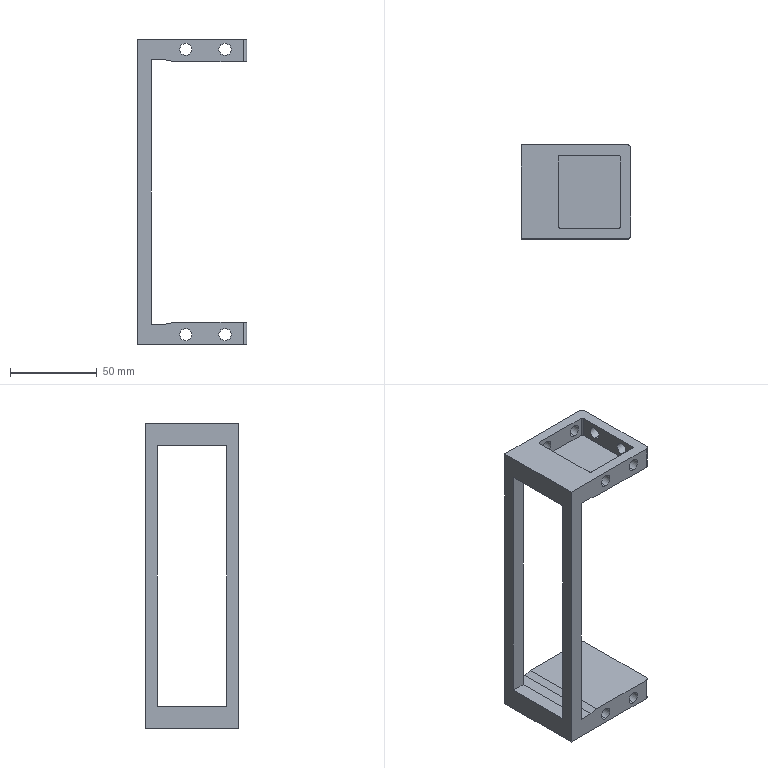Part | STEP file | TKR26H40W150R75+18L-FU-MU-Part-2 | 1 solid | 64 faces | box 63 x 54 x 176 mm | volume 65545 mm3 | cylinder 36 | plane 28 | commonest cylinder face diameters 7 x24 2 x8 4 x4